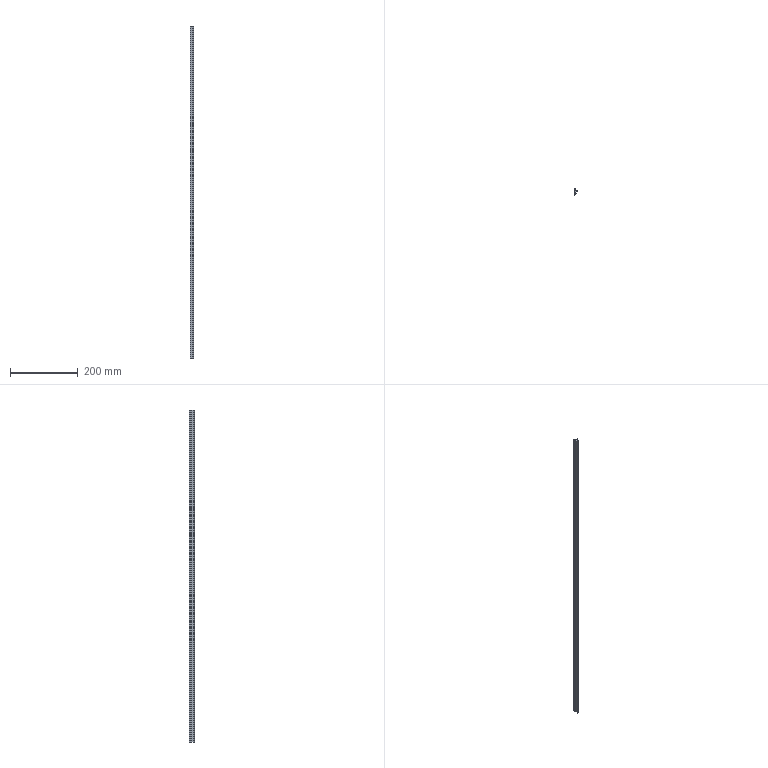Part | SolidWorks | features BaseBody 1, MoveFace 1 | 1 solid | 20 faces | box 10.8 x 17.5 x 980 mm | volume 77225 mm3 | cylinder 11 | plane 9 | commonest cylinder face diameters 1.6 x2 14 x2 0.4 x1 0.6 x1 0.8 x1 2.6 x1
STEP:
#1=CARTESIAN_POINT('',(-3.236,-11.055,880.));
#2=VERTEX_POINT('',#1);
#3=CARTESIAN_POINT('',(-4.3,-10.3,880.));
#4=VERTEX_POINT('',#3);
#5=CARTESIAN_POINT('',(-3.5,-10.3,880.));
#6=DIRECTION('',(0.,0.,-1.));
#7=DIRECTION('',(1.,0.,0.));
#8=AXIS2_PLACEMENT_3D('',#5,#6,#7);
#9=CIRCLE('',#8,0.8);
#10=EDGE_CURVE('',#2,#4,#9,.T.);
#11=ORIENTED_EDGE('',*,*,#10,.T.);
#12=CARTESIAN_POINT('',(-4.3,-10.3,-100.));
#13=VERTEX_POINT('',#12);
#14=CARTESIAN_POINT('',(-4.3,-10.3,-100.));
#15=DIRECTION('',(0.,0.,-1.));
#16=VECTOR('',#15,1000.);
#17=LINE('',#14,#16);
#18=EDGE_CURVE('',#4,#13,#17,.T.);
#19=ORIENTED_EDGE('',*,*,#18,.T.);
#20=CARTESIAN_POINT('',(-3.236,-11.055,-100.));
#21=VERTEX_POINT('',#20);
#22=CARTESIAN_POINT('',(-3.5,-10.3,-100.));
#23=DIRECTION('',(0.,0.,1.));
#24=DIRECTION('',(-1.,0.,0.));
#25=AXIS2_PLACEMENT_3D('',#22,#23,#24);
#26=CIRCLE('',#25,0.8);
#27=EDGE_CURVE('',#13,#21,#26,.T.);
#28=ORIENTED_EDGE('',*,*,#27,.T.);
#29=CARTESIAN_POINT('',(-3.236,-11.055,-100.));
#30=DIRECTION('',(0.,0.,-1.));
#31=VECTOR('',#30,1000.);
#32=LINE('',#29,#31);
#33=EDGE_CURVE('',#2,#21,#32,.T.);
#34=ORIENTED_EDGE('',*,*,#33,.F.);
#35=EDGE_LOOP('',(#11,#19,#28,#34));
#36=FACE_OUTER_BOUND('',#35,.T.);
#37=CARTESIAN_POINT('',(-3.5,-10.3,-100.));
#38=DIRECTION('',(0.,0.,-1.));
#39=DIRECTION('',(-1.,0.,0.));
#40=AXIS2_PLACEMENT_3D('',#37,#38,#39);
#41=CYLINDRICAL_SURFACE('',#40,0.8);
#42=ADVANCED_FACE('',(#36),#41,.T.);
#43=CARTESIAN_POINT('',(1.184,-6.397,-100.));
#44=VERTEX_POINT('',#43);
#45=CARTESIAN_POINT('',(-5.702,-4.29,-100.));
#46=DIRECTION('',(0.,0.,1.));
#47=DIRECTION('',(-1.,0.,0.));
#48=AXIS2_PLACEMENT_3D('',#45,#46,#47);
#49=CIRCLE('',#48,7.201);
#50=EDGE_CURVE('',#21,#44,#49,.T.);
#51=ORIENTED_EDGE('',*,*,#50,.T.);
#52=CARTESIAN_POINT('',(1.184,-6.397,880.));
#53=VERTEX_POINT('',#52);
#54=CARTESIAN_POINT('',(1.184,-6.397,-100.));
#55=DIRECTION('',(0.,0.,1.));
#56=VECTOR('',#55,1000.);
#57=LINE('',#54,#56);
#58=EDGE_CURVE('',#44,#53,#57,.T.);
#59=ORIENTED_EDGE('',*,*,#58,.T.);
#60=CARTESIAN_POINT('',(-5.702,-4.29,880.));
#61=DIRECTION('',(0.,0.,-1.));
#62=DIRECTION('',(1.,0.,0.));
#63=AXIS2_PLACEMENT_3D('',#60,#61,#62);
#64=CIRCLE('',#63,7.201);
#65=EDGE_CURVE('',#53,#2,#64,.T.);
#66=ORIENTED_EDGE('',*,*,#65,.T.);
#67=ORIENTED_EDGE('',*,*,#33,.T.);
#68=EDGE_LOOP('',(#51,#59,#66,#67));
#69=FACE_OUTER_BOUND('',#68,.T.);
#70=CARTESIAN_POINT('',(-5.702,-4.29,-100.));
#71=DIRECTION('',(0.,0.,-1.));
#72=DIRECTION('',(-1.,0.,0.));
#73=AXIS2_PLACEMENT_3D('',#70,#71,#72);
#74=CYLINDRICAL_SURFACE('',#73,7.201);
#75=ADVANCED_FACE('',(#69),#74,.T.);
#76=CARTESIAN_POINT('',(0.9,-6.,-100.));
#77=VERTEX_POINT('',#76);
#78=CARTESIAN_POINT('',(0.9,-6.3,-100.));
#79=DIRECTION('',(0.,0.,1.));
#80=DIRECTION('',(-1.,0.,0.));
#81=AXIS2_PLACEMENT_3D('',#78,#79,#80);
#82=CIRCLE('',#81,0.3);
#83=EDGE_CURVE('',#44,#77,#82,.T.);
#84=ORIENTED_EDGE('',*,*,#83,.T.);
#85=CARTESIAN_POINT('',(0.9,-6.,880.));
#86=VERTEX_POINT('',#85);
#87=CARTESIAN_POINT('',(0.9,-6.,-100.));
#88=DIRECTION('',(0.,0.,1.));
#89=VECTOR('',#88,1000.);
#90=LINE('',#87,#89);
#91=EDGE_CURVE('',#77,#86,#90,.T.);
#92=ORIENTED_EDGE('',*,*,#91,.T.);
#93=CARTESIAN_POINT('',(0.9,-6.3,880.));
#94=DIRECTION('',(0.,0.,-1.));
#95=DIRECTION('',(1.,0.,0.));
#96=AXIS2_PLACEMENT_3D('',#93,#94,#95);
#97=CIRCLE('',#96,0.3);
#98=EDGE_CURVE('',#86,#53,#97,.T.);
#99=ORIENTED_EDGE('',*,*,#98,.T.);
#100=ORIENTED_EDGE('',*,*,#58,.F.);
#101=EDGE_LOOP('',(#84,#92,#99,#100));
#102=FACE_OUTER_BOUND('',#101,.T.);
#103=CARTESIAN_POINT('',(0.9,-6.3,-100.));
#104=DIRECTION('',(0.,0.,-1.));
#105=DIRECTION('',(-1.,0.,0.));
#106=AXIS2_PLACEMENT_3D('',#103,#104,#105);
#107=CYLINDRICAL_SURFACE('',#106,0.3);
#108=ADVANCED_FACE('',(#102),#107,.T.);
#109=CARTESIAN_POINT('',(-2.5,-0.5,-100.));
#110=VERTEX_POINT('',#109);
#111=CARTESIAN_POINT('',(-2.5,-6.153,-100.));
#112=VERTEX_POINT('',#111);
#113=CARTESIAN_POINT('',(-2.5,-6.397,-100.));
#114=DIRECTION('',(0.,-1.,0.));
#115=VECTOR('',#114,1000.);
#116=LINE('',#113,#115);
#117=EDGE_CURVE('',#110,#112,#116,.T.);
#118=ORIENTED_EDGE('',*,*,#117,.F.);
#119=CARTESIAN_POINT('',(-4.2,1.695,-100.));
#120=VERTEX_POINT('',#119);
#121=CARTESIAN_POINT('',(-1.701,1.875,-100.));
#122=DIRECTION('',(0.,0.,1.));
#123=DIRECTION('',(-1.,0.,0.));
#124=AXIS2_PLACEMENT_3D('',#121,#122,#123);
#125=CIRCLE('',#124,2.506);
#126=EDGE_CURVE('',#120,#110,#125,.T.);
#127=ORIENTED_EDGE('',*,*,#126,.F.);
#128=CARTESIAN_POINT('',(-4.2,5.1,-100.));
#129=VERTEX_POINT('',#128);
#130=CARTESIAN_POINT('',(-4.2,-6.397,-100.));
#131=DIRECTION('',(0.,-1.,0.));
#132=VECTOR('',#131,1000.);
#133=LINE('',#130,#132);
#134=EDGE_CURVE('',#129,#120,#133,.T.);
#135=ORIENTED_EDGE('',*,*,#134,.F.);
#136=CARTESIAN_POINT('',(-2.892,6.4,-100.));
#137=VERTEX_POINT('',#136);
#138=CARTESIAN_POINT('',(-2.9,5.1,-100.));
#139=DIRECTION('',(0.,0.,1.));
#140=DIRECTION('',(-1.,0.,0.));
#141=AXIS2_PLACEMENT_3D('',#138,#139,#140);
#142=CIRCLE('',#141,1.3);
#143=EDGE_CURVE('',#137,#129,#142,.T.);
#144=ORIENTED_EDGE('',*,*,#143,.F.);
#145=CARTESIAN_POINT('',(0.5,5.5,-100.));
#146=VERTEX_POINT('',#145);
#147=CARTESIAN_POINT('',(-2.934,-0.5999,-100.));
#148=DIRECTION('',(0.,0.,1.));
#149=DIRECTION('',(-1.,0.,0.));
#150=AXIS2_PLACEMENT_3D('',#147,#148,#149);
#151=CIRCLE('',#150,7.);
#152=EDGE_CURVE('',#146,#137,#151,.T.);
#153=ORIENTED_EDGE('',*,*,#152,.F.);
#154=CARTESIAN_POINT('',(5.5,1.7,-100.));
#155=VERTEX_POINT('',#154);
#156=CARTESIAN_POINT('',(5.5,1.7,-100.));
#157=DIRECTION('',(-0.7962,0.6051,0.));
#158=VECTOR('',#157,1000.);
#159=LINE('',#156,#158);
#160=EDGE_CURVE('',#155,#146,#159,.T.);
#161=ORIENTED_EDGE('',*,*,#160,.F.);
#162=CARTESIAN_POINT('',(6.458,-0.2215,-100.));
#163=VERTEX_POINT('',#162);
#164=CARTESIAN_POINT('',(6.458,-0.2215,-100.));
#165=DIRECTION('',(-0.4462,0.8949,0.));
#166=VECTOR('',#165,1000.);
#167=LINE('',#164,#166);
#168=EDGE_CURVE('',#163,#155,#167,.T.);
#169=ORIENTED_EDGE('',*,*,#168,.F.);
#170=CARTESIAN_POINT('',(5.895,-0.7433,-100.));
#171=VERTEX_POINT('',#170);
#172=CARTESIAN_POINT('',(6.1,-0.4,-100.));
#173=DIRECTION('',(0.,0.,1.));
#174=DIRECTION('',(-1.,0.,0.));
#175=AXIS2_PLACEMENT_3D('',#172,#173,#174);
#176=CIRCLE('',#175,0.4);
#177=EDGE_CURVE('',#171,#163,#176,.T.);
#178=ORIENTED_EDGE('',*,*,#177,.F.);
#179=CARTESIAN_POINT('',(3.,0.,-100.));
#180=VERTEX_POINT('',#179);
#181=CARTESIAN_POINT('',(2.746,-6.995,-100.));
#182=DIRECTION('',(0.,0.,-1.));
#183=DIRECTION('',(-1.,0.,0.));
#184=AXIS2_PLACEMENT_3D('',#181,#182,#183);
#185=CIRCLE('',#184,7.);
#186=EDGE_CURVE('',#180,#171,#185,.T.);
#187=ORIENTED_EDGE('',*,*,#186,.F.);
#188=CARTESIAN_POINT('',(0.,0.,-100.));
#189=VERTEX_POINT('',#188);
#190=CARTESIAN_POINT('',(-6.814,0.,-100.));
#191=DIRECTION('',(1.,0.,0.));
#192=VECTOR('',#191,1000.);
#193=LINE('',#190,#192);
#194=EDGE_CURVE('',#189,#180,#193,.T.);
#195=ORIENTED_EDGE('',*,*,#194,.F.);
#196=CARTESIAN_POINT('',(0.,-5.8,-100.));
#197=VERTEX_POINT('',#196);
#198=CARTESIAN_POINT('',(0.,-6.397,-100.));
#199=DIRECTION('',(0.,1.,0.));
#200=VECTOR('',#199,1000.);
#201=LINE('',#198,#200);
#202=EDGE_CURVE('',#197,#189,#201,.T.);
#203=ORIENTED_EDGE('',*,*,#202,.F.);
#204=CARTESIAN_POINT('',(0.2,-6.,-100.));
#205=VERTEX_POINT('',#204);
#206=CARTESIAN_POINT('',(0.2,-5.8,-100.));
#207=DIRECTION('',(0.,0.,1.));
#208=DIRECTION('',(-1.,0.,0.));
#209=AXIS2_PLACEMENT_3D('',#206,#207,#208);
#210=CIRCLE('',#209,0.2);
#211=EDGE_CURVE('',#197,#205,#210,.T.);
#212=ORIENTED_EDGE('',*,*,#211,.T.);
#213=CARTESIAN_POINT('',(-6.814,-6.,-100.));
#214=DIRECTION('',(-1.,0.,0.));
#215=VECTOR('',#214,1000.);
#216=LINE('',#213,#215);
#217=EDGE_CURVE('',#77,#205,#216,.T.);
#218=ORIENTED_EDGE('',*,*,#217,.F.);
#219=ORIENTED_EDGE('',*,*,#83,.F.);
#220=ORIENTED_EDGE('',*,*,#50,.F.);
#221=ORIENTED_EDGE('',*,*,#27,.F.);
#222=CARTESIAN_POINT('',(-3.998,-9.674,-100.));
#223=VERTEX_POINT('',#222);
#224=CARTESIAN_POINT('',(-3.5,-10.3,-100.));
#225=DIRECTION('',(0.,0.,1.));
#226=DIRECTION('',(-1.,0.,0.));
#227=AXIS2_PLACEMENT_3D('',#224,#225,#226);
#228=CIRCLE('',#227,0.8);
#229=EDGE_CURVE('',#223,#13,#228,.T.);
#230=ORIENTED_EDGE('',*,*,#229,.F.);
#231=CARTESIAN_POINT('',(-6.814,-6.397,-100.));
#232=DIRECTION('',(0.,0.,-1.));
#233=DIRECTION('',(-1.,0.,0.));
#234=AXIS2_PLACEMENT_3D('',#231,#232,#233);
#235=CIRCLE('',#234,4.321);
#236=EDGE_CURVE('',#112,#223,#235,.T.);
#237=ORIENTED_EDGE('',*,*,#236,.F.);
#238=EDGE_LOOP('',(#118,#127,#135,#144,#153,#161,#169,#178,#187,#195,#203,#212,#218,#219,#220,#221,#230,#237));
#239=FACE_OUTER_BOUND('',#238,.T.);
#240=CARTESIAN_POINT('',(-6.814,-6.397,-100.));
#241=DIRECTION('',(0.,0.,1.));
#242=DIRECTION('',(1.,0.,0.));
#243=AXIS2_PLACEMENT_3D('',#240,#241,#242);
#244=PLANE('',#243);
#245=ADVANCED_FACE('',(#239),#244,.F.);
#246=ORIENTED_EDGE('',*,*,#18,.F.);
#247=CARTESIAN_POINT('',(-3.998,-9.674,880.));
#248=VERTEX_POINT('',#247);
#249=CARTESIAN_POINT('',(-3.5,-10.3,880.));
#250=DIRECTION('',(0.,0.,-1.));
#251=DIRECTION('',(1.,0.,0.));
#252=AXIS2_PLACEMENT_3D('',#249,#250,#251);
#253=CIRCLE('',#252,0.8);
#254=EDGE_CURVE('',#4,#248,#253,.T.);
#255=ORIENTED_EDGE('',*,*,#254,.T.);
#256=CARTESIAN_POINT('',(-3.998,-9.674,-100.));
#257=DIRECTION('',(0.,0.,-1.));
#258=VECTOR('',#257,1000.);
#259=LINE('',#256,#258);
#260=EDGE_CURVE('',#248,#223,#259,.T.);
#261=ORIENTED_EDGE('',*,*,#260,.T.);
#262=ORIENTED_EDGE('',*,*,#229,.T.);
#263=EDGE_LOOP('',(#246,#255,#261,#262));
#264=FACE_OUTER_BOUND('',#263,.T.);
#265=CARTESIAN_POINT('',(-3.5,-10.3,-100.));
#266=DIRECTION('',(0.,0.,-1.));
#267=DIRECTION('',(-1.,0.,0.));
#268=AXIS2_PLACEMENT_3D('',#265,#266,#267);
#269=CYLINDRICAL_SURFACE('',#268,0.8);
#270=ADVANCED_FACE('',(#264),#269,.T.);
#271=CARTESIAN_POINT('',(-4.2,1.695,880.));
#272=VERTEX_POINT('',#271);
#273=CARTESIAN_POINT('',(-2.5,-0.5,880.));
#274=VERTEX_POINT('',#273);
#275=CARTESIAN_POINT('',(-1.701,1.875,880.));
#276=DIRECTION('',(0.,0.,1.));
#277=DIRECTION('',(1.,0.,0.));
#278=AXIS2_PLACEMENT_3D('',#275,#276,#277);
#279=CIRCLE('',#278,2.506);
#280=EDGE_CURVE('',#272,#274,#279,.T.);
#281=ORIENTED_EDGE('',*,*,#280,.T.);
#282=CARTESIAN_POINT('',(-2.5,-6.153,880.));
#283=VERTEX_POINT('',#282);
#284=CARTESIAN_POINT('',(-2.5,-6.397,880.));
#285=DIRECTION('',(0.,-1.,0.));
#286=VECTOR('',#285,1000.);
#287=LINE('',#284,#286);
#288=EDGE_CURVE('',#274,#283,#287,.T.);
#289=ORIENTED_EDGE('',*,*,#288,.T.);
#290=CARTESIAN_POINT('',(-6.814,-6.397,880.));
#291=DIRECTION('',(0.,0.,-1.));
#292=DIRECTION('',(1.,0.,0.));
#293=AXIS2_PLACEMENT_3D('',#290,#291,#292);
#294=CIRCLE('',#293,4.321);
#295=EDGE_CURVE('',#283,#248,#294,.T.);
#296=ORIENTED_EDGE('',*,*,#295,.T.);
#297=ORIENTED_EDGE('',*,*,#254,.F.);
#298=ORIENTED_EDGE('',*,*,#10,.F.);
#299=ORIENTED_EDGE('',*,*,#65,.F.);
#300=ORIENTED_EDGE('',*,*,#98,.F.);
#301=CARTESIAN_POINT('',(0.2,-6.,880.));
#302=VERTEX_POINT('',#301);
#303=CARTESIAN_POINT('',(-6.814,-6.,880.));
#304=DIRECTION('',(-1.,0.,0.));
#305=VECTOR('',#304,1000.);
#306=LINE('',#303,#305);
#307=EDGE_CURVE('',#86,#302,#306,.T.);
#308=ORIENTED_EDGE('',*,*,#307,.T.);
#309=CARTESIAN_POINT('',(0.,-5.8,880.));
#310=VERTEX_POINT('',#309);
#311=CARTESIAN_POINT('',(0.2,-5.8,880.));
#312=DIRECTION('',(0.,0.,-1.));
#313=DIRECTION('',(1.,0.,0.));
#314=AXIS2_PLACEMENT_3D('',#311,#312,#313);
#315=CIRCLE('',#314,0.2);
#316=EDGE_CURVE('',#302,#310,#315,.T.);
#317=ORIENTED_EDGE('',*,*,#316,.T.);
#318=CARTESIAN_POINT('',(0.,0.,880.));
#319=VERTEX_POINT('',#318);
#320=CARTESIAN_POINT('',(0.,-6.397,880.));
#321=DIRECTION('',(0.,1.,0.));
#322=VECTOR('',#321,1000.);
#323=LINE('',#320,#322);
#324=EDGE_CURVE('',#310,#319,#323,.T.);
#325=ORIENTED_EDGE('',*,*,#324,.T.);
#326=CARTESIAN_POINT('',(3.,0.,880.));
#327=VERTEX_POINT('',#326);
#328=CARTESIAN_POINT('',(-6.814,0.,880.));
#329=DIRECTION('',(1.,0.,0.));
#330=VECTOR('',#329,1000.);
#331=LINE('',#328,#330);
#332=EDGE_CURVE('',#319,#327,#331,.T.);
#333=ORIENTED_EDGE('',*,*,#332,.T.);
#334=CARTESIAN_POINT('',(5.895,-0.7433,880.));
#335=VERTEX_POINT('',#334);
#336=CARTESIAN_POINT('',(2.746,-6.995,880.));
#337=DIRECTION('',(0.,0.,-1.));
#338=DIRECTION('',(1.,0.,0.));
#339=AXIS2_PLACEMENT_3D('',#336,#337,#338);
#340=CIRCLE('',#339,7.);
#341=EDGE_CURVE('',#327,#335,#340,.T.);
#342=ORIENTED_EDGE('',*,*,#341,.T.);
#343=CARTESIAN_POINT('',(6.458,-0.2215,880.));
#344=VERTEX_POINT('',#343);
#345=CARTESIAN_POINT('',(6.1,-0.4,880.));
#346=DIRECTION('',(0.,0.,-1.));
#347=DIRECTION('',(1.,0.,0.));
#348=AXIS2_PLACEMENT_3D('',#345,#346,#347);
#349=CIRCLE('',#348,0.4);
#350=EDGE_CURVE('',#344,#335,#349,.T.);
#351=ORIENTED_EDGE('',*,*,#350,.F.);
#352=CARTESIAN_POINT('',(5.5,1.7,880.));
#353=VERTEX_POINT('',#352);
#354=CARTESIAN_POINT('',(6.282,0.1323,880.));
#355=DIRECTION('',(-0.4462,0.8949,0.));
#356=VECTOR('',#355,1000.);
#357=LINE('',#354,#356);
#358=EDGE_CURVE('',#344,#353,#357,.T.);
#359=ORIENTED_EDGE('',*,*,#358,.T.);
#360=CARTESIAN_POINT('',(0.5,5.5,880.));
#361=VERTEX_POINT('',#360);
#362=CARTESIAN_POINT('',(1.595,4.668,880.));
#363=DIRECTION('',(-0.7962,0.6051,0.));
#364=VECTOR('',#363,1000.);
#365=LINE('',#362,#364);
#366=EDGE_CURVE('',#353,#361,#365,.T.);
#367=ORIENTED_EDGE('',*,*,#366,.T.);
#368=CARTESIAN_POINT('',(-2.892,6.4,880.));
#369=VERTEX_POINT('',#368);
#370=CARTESIAN_POINT('',(-2.934,-0.5999,880.));
#371=DIRECTION('',(0.,0.,1.));
#372=DIRECTION('',(1.,0.,0.));
#373=AXIS2_PLACEMENT_3D('',#370,#371,#372);
#374=CIRCLE('',#373,7.);
#375=EDGE_CURVE('',#361,#369,#374,.T.);
#376=ORIENTED_EDGE('',*,*,#375,.T.);
#377=CARTESIAN_POINT('',(-4.2,5.1,880.));
#378=VERTEX_POINT('',#377);
#379=CARTESIAN_POINT('',(-2.9,5.1,880.));
#380=DIRECTION('',(0.,0.,1.));
#381=DIRECTION('',(1.,0.,0.));
#382=AXIS2_PLACEMENT_3D('',#379,#380,#381);
#383=CIRCLE('',#382,1.3);
#384=EDGE_CURVE('',#369,#378,#383,.T.);
#385=ORIENTED_EDGE('',*,*,#384,.T.);
#386=CARTESIAN_POINT('',(-4.2,-6.397,880.));
#387=DIRECTION('',(0.,-1.,0.));
#388=VECTOR('',#387,1000.);
#389=LINE('',#386,#388);
#390=EDGE_CURVE('',#378,#272,#389,.T.);
#391=ORIENTED_EDGE('',*,*,#390,.T.);
#392=EDGE_LOOP('',(#281,#289,#296,#297,#298,#299,#300,#308,#317,#325,#333,#342,#351,#359,#367,#376,#385,#391));
#393=FACE_OUTER_BOUND('',#392,.T.);
#394=CARTESIAN_POINT('',(-6.814,-6.397,880.));
#395=DIRECTION('',(0.,0.,1.));
#396=DIRECTION('',(1.,0.,0.));
#397=AXIS2_PLACEMENT_3D('',#394,#395,#396);
#398=PLANE('',#397);
#399=ADVANCED_FACE('',(#393),#398,.T.);
#400=ORIENTED_EDGE('',*,*,#217,.T.);
#401=CARTESIAN_POINT('',(0.2,-6.,-100.));
#402=DIRECTION('',(0.,0.,1.));
#403=VECTOR('',#402,1000.);
#404=LINE('',#401,#403);
#405=EDGE_CURVE('',#205,#302,#404,.T.);
#406=ORIENTED_EDGE('',*,*,#405,.T.);
#407=ORIENTED_EDGE('',*,*,#307,.F.);
#408=ORIENTED_EDGE('',*,*,#91,.F.);
#409=EDGE_LOOP('',(#400,#406,#407,#408));
#410=FACE_OUTER_BOUND('',#409,.T.);
#411=CARTESIAN_POINT('',(0.9,-6.,-100.));
#412=DIRECTION('',(0.,1.,0.));
#413=DIRECTION('',(0.,0.,1.));
#414=AXIS2_PLACEMENT_3D('',#411,#412,#413);
#415=PLANE('',#414);
#416=ADVANCED_FACE('',(#410),#415,.T.);
#417=CARTESIAN_POINT('',(-2.5,-6.153,-100.));
#418=DIRECTION('',(0.,0.,1.));
#419=VECTOR('',#418,1000.);
#420=LINE('',#417,#419);
#421=EDGE_CURVE('',#112,#283,#420,.T.);
#422=ORIENTED_EDGE('',*,*,#421,.F.);
#423=ORIENTED_EDGE('',*,*,#236,.T.);
#424=ORIENTED_EDGE('',*,*,#260,.F.);
#425=ORIENTED_EDGE('',*,*,#295,.F.);
#426=EDGE_LOOP('',(#422,#423,#424,#425));
#427=FACE_OUTER_BOUND('',#426,.T.);
#428=CARTESIAN_POINT('',(-6.814,-6.397,-100.));
#429=DIRECTION('',(0.,0.,-1.));
#430=DIRECTION('',(-1.,0.,0.));
#431=AXIS2_PLACEMENT_3D('',#428,#429,#430);
#432=CYLINDRICAL_SURFACE('',#431,4.321);
#433=ADVANCED_FACE('',(#427),#432,.F.);
#434=ORIENTED_EDGE('',*,*,#117,.T.);
#435=ORIENTED_EDGE('',*,*,#421,.T.);
#436=ORIENTED_EDGE('',*,*,#288,.F.);
#437=CARTESIAN_POINT('',(-2.5,-0.5,-100.));
#438=DIRECTION('',(0.,0.,-1.));
#439=VECTOR('',#438,1000.);
#440=LINE('',#437,#439);
#441=EDGE_CURVE('',#274,#110,#440,.T.);
#442=ORIENTED_EDGE('',*,*,#441,.T.);
#443=EDGE_LOOP('',(#434,#435,#436,#442));
#444=FACE_OUTER_BOUND('',#443,.T.);
#445=CARTESIAN_POINT('',(-2.5,-0.5,-100.));
#446=DIRECTION('',(-1.,0.,0.));
#447=DIRECTION('',(0.,0.,1.));
#448=AXIS2_PLACEMENT_3D('',#445,#446,#447);
#449=PLANE('',#448);
#450=ADVANCED_FACE('',(#444),#449,.T.);
#451=ORIENTED_EDGE('',*,*,#126,.T.);
#452=ORIENTED_EDGE('',*,*,#441,.F.);
#453=ORIENTED_EDGE('',*,*,#280,.F.);
#454=CARTESIAN_POINT('',(-4.2,1.695,-100.));
#455=DIRECTION('',(0.,0.,-1.));
#456=VECTOR('',#455,1000.);
#457=LINE('',#454,#456);
#458=EDGE_CURVE('',#272,#120,#457,.T.);
#459=ORIENTED_EDGE('',*,*,#458,.T.);
#460=EDGE_LOOP('',(#451,#452,#453,#459));
#461=FACE_OUTER_BOUND('',#460,.T.);
#462=CARTESIAN_POINT('',(-1.701,1.875,-100.));
#463=DIRECTION('',(0.,0.,-1.));
#464=DIRECTION('',(-1.,0.,0.));
#465=AXIS2_PLACEMENT_3D('',#462,#463,#464);
#466=CYLINDRICAL_SURFACE('',#465,2.506);
#467=ADVANCED_FACE('',(#461),#466,.T.);
#468=ORIENTED_EDGE('',*,*,#134,.T.);
#469=ORIENTED_EDGE('',*,*,#458,.F.);
#470=ORIENTED_EDGE('',*,*,#390,.F.);
#471=CARTESIAN_POINT('',(-4.2,5.1,-100.));
#472=DIRECTION('',(0.,0.,-1.));
#473=VECTOR('',#472,1000.);
#474=LINE('',#471,#473);
#475=EDGE_CURVE('',#378,#129,#474,.T.);
#476=ORIENTED_EDGE('',*,*,#475,.T.);
#477=EDGE_LOOP('',(#468,#469,#470,#476));
#478=FACE_OUTER_BOUND('',#477,.T.);
#479=CARTESIAN_POINT('',(-4.2,5.1,-100.));
#480=DIRECTION('',(-1.,0.,0.));
#481=DIRECTION('',(0.,0.,1.));
#482=AXIS2_PLACEMENT_3D('',#479,#480,#481);
#483=PLANE('',#482);
#484=ADVANCED_FACE('',(#478),#483,.T.);
#485=ORIENTED_EDGE('',*,*,#143,.T.);
#486=ORIENTED_EDGE('',*,*,#475,.F.);
#487=ORIENTED_EDGE('',*,*,#384,.F.);
#488=CARTESIAN_POINT('',(-2.892,6.4,-100.));
#489=DIRECTION('',(0.,0.,-1.));
#490=VECTOR('',#489,1000.);
#491=LINE('',#488,#490);
#492=EDGE_CURVE('',#369,#137,#491,.T.);
#493=ORIENTED_EDGE('',*,*,#492,.T.);
#494=EDGE_LOOP('',(#485,#486,#487,#493));
#495=FACE_OUTER_BOUND('',#494,.T.);
#496=CARTESIAN_POINT('',(-2.9,5.1,-100.));
#497=DIRECTION('',(0.,0.,-1.));
#498=DIRECTION('',(-1.,0.,0.));
#499=AXIS2_PLACEMENT_3D('',#496,#497,#498);
#500=CYLINDRICAL_SURFACE('',#499,1.3);
#501=ADVANCED_FACE('',(#495),#500,.T.);
#502=ORIENTED_EDGE('',*,*,#152,.T.);
#503=ORIENTED_EDGE('',*,*,#492,.F.);
#504=ORIENTED_EDGE('',*,*,#375,.F.);
#505=CARTESIAN_POINT('',(0.5,5.5,-100.));
#506=DIRECTION('',(0.,0.,-1.));
#507=VECTOR('',#506,1000.);
#508=LINE('',#505,#507);
#509=EDGE_CURVE('',#361,#146,#508,.T.);
#510=ORIENTED_EDGE('',*,*,#509,.T.);
#511=EDGE_LOOP('',(#502,#503,#504,#510));
#512=FACE_OUTER_BOUND('',#511,.T.);
#513=CARTESIAN_POINT('',(-2.934,-0.5999,-100.));
#514=DIRECTION('',(0.,0.,-1.));
#515=DIRECTION('',(-1.,0.,0.));
#516=AXIS2_PLACEMENT_3D('',#513,#514,#515);
#517=CYLINDRICAL_SURFACE('',#516,7.);
#518=ADVANCED_FACE('',(#512),#517,.T.);
#519=ORIENTED_EDGE('',*,*,#160,.T.);
#520=ORIENTED_EDGE('',*,*,#509,.F.);
#521=ORIENTED_EDGE('',*,*,#366,.F.);
#522=CARTESIAN_POINT('',(5.5,1.7,-100.));
#523=DIRECTION('',(0.,0.,-1.));
#524=VECTOR('',#523,1000.);
#525=LINE('',#522,#524);
#526=EDGE_CURVE('',#353,#155,#525,.T.);
#527=ORIENTED_EDGE('',*,*,#526,.T.);
#528=EDGE_LOOP('',(#519,#520,#521,#527));
#529=FACE_OUTER_BOUND('',#528,.T.);
#530=CARTESIAN_POINT('',(5.5,1.7,-100.));
#531=DIRECTION('',(0.6051,0.7962,0.));
#532=DIRECTION('',(-0.7962,0.6051,0.));
#533=AXIS2_PLACEMENT_3D('',#530,#531,#532);
#534=PLANE('',#533);
#535=ADVANCED_FACE('',(#529),#534,.T.);
#536=ORIENTED_EDGE('',*,*,#168,.T.);
#537=ORIENTED_EDGE('',*,*,#526,.F.);
#538=ORIENTED_EDGE('',*,*,#358,.F.);
#539=CARTESIAN_POINT('',(6.458,-0.2215,-100.));
#540=DIRECTION('',(0.,0.,-1.));
#541=VECTOR('',#540,1000.);
#542=LINE('',#539,#541);
#543=EDGE_CURVE('',#344,#163,#542,.T.);
#544=ORIENTED_EDGE('',*,*,#543,.T.);
#545=EDGE_LOOP('',(#536,#537,#538,#544));
#546=FACE_OUTER_BOUND('',#545,.T.);
#547=CARTESIAN_POINT('',(6.458,-0.2215,-100.));
#548=DIRECTION('',(0.8949,0.4462,0.));
#549=DIRECTION('',(-0.4462,0.8949,0.));
#550=AXIS2_PLACEMENT_3D('',#547,#548,#549);
#551=PLANE('',#550);
#552=ADVANCED_FACE('',(#546),#551,.T.);
#553=CARTESIAN_POINT('',(3.,0.,-100.));
#554=DIRECTION('',(0.,0.,1.));
#555=VECTOR('',#554,1000.);
#556=LINE('',#553,#555);
#557=EDGE_CURVE('',#180,#327,#556,.T.);
#558=ORIENTED_EDGE('',*,*,#557,.F.);
#559=ORIENTED_EDGE('',*,*,#186,.T.);
#560=CARTESIAN_POINT('',(5.895,-0.7433,-100.));
#561=DIRECTION('',(0.,0.,-1.));
#562=VECTOR('',#561,1000.);
#563=LINE('',#560,#562);
#564=EDGE_CURVE('',#335,#171,#563,.T.);
#565=ORIENTED_EDGE('',*,*,#564,.F.);
#566=ORIENTED_EDGE('',*,*,#341,.F.);
#567=EDGE_LOOP('',(#558,#559,#565,#566));
#568=FACE_OUTER_BOUND('',#567,.T.);
#569=CARTESIAN_POINT('',(2.746,-6.995,-100.));
#570=DIRECTION('',(0.,0.,-1.));
#571=DIRECTION('',(-1.,0.,0.));
#572=AXIS2_PLACEMENT_3D('',#569,#570,#571);
#573=CYLINDRICAL_SURFACE('',#572,7.);
#574=ADVANCED_FACE('',(#568),#573,.F.);
#575=ORIENTED_EDGE('',*,*,#194,.T.);
#576=ORIENTED_EDGE('',*,*,#557,.T.);
#577=ORIENTED_EDGE('',*,*,#332,.F.);
#578=CARTESIAN_POINT('',(0.,0.,-100.));
#579=DIRECTION('',(0.,0.,-1.));
#580=VECTOR('',#579,1000.);
#581=LINE('',#578,#580);
#582=EDGE_CURVE('',#319,#189,#581,.T.);
#583=ORIENTED_EDGE('',*,*,#582,.T.);
#584=EDGE_LOOP('',(#575,#576,#577,#583));
#585=FACE_OUTER_BOUND('',#584,.T.);
#586=CARTESIAN_POINT('',(0.,0.,-100.));
#587=DIRECTION('',(0.,-1.,0.));
#588=DIRECTION('',(0.,0.,-1.));
#589=AXIS2_PLACEMENT_3D('',#586,#587,#588);
#590=PLANE('',#589);
#591=ADVANCED_FACE('',(#585),#590,.T.);
#592=ORIENTED_EDGE('',*,*,#202,.T.);
#593=ORIENTED_EDGE('',*,*,#582,.F.);
#594=ORIENTED_EDGE('',*,*,#324,.F.);
#595=CARTESIAN_POINT('',(0.,-5.8,-100.));
#596=DIRECTION('',(0.,0.,-1.));
#597=VECTOR('',#596,1000.);
#598=LINE('',#595,#597);
#599=EDGE_CURVE('',#310,#197,#598,.T.);
#600=ORIENTED_EDGE('',*,*,#599,.T.);
#601=EDGE_LOOP('',(#592,#593,#594,#600));
#602=FACE_OUTER_BOUND('',#601,.T.);
#603=CARTESIAN_POINT('',(0.,-5.8,-100.));
#604=DIRECTION('',(1.,0.,0.));
#605=DIRECTION('',(0.,0.,-1.));
#606=AXIS2_PLACEMENT_3D('',#603,#604,#605);
#607=PLANE('',#606);
#608=ADVANCED_FACE('',(#602),#607,.T.);
#609=ORIENTED_EDGE('',*,*,#405,.F.);
#610=ORIENTED_EDGE('',*,*,#211,.F.);
#611=ORIENTED_EDGE('',*,*,#599,.F.);
#612=ORIENTED_EDGE('',*,*,#316,.F.);
#613=EDGE_LOOP('',(#609,#610,#611,#612));
#614=FACE_OUTER_BOUND('',#613,.T.);
#615=CARTESIAN_POINT('',(0.2,-5.8,-100.));
#616=DIRECTION('',(0.,0.,-1.));
#617=DIRECTION('',(-1.,0.,0.));
#618=AXIS2_PLACEMENT_3D('',#615,#616,#617);
#619=CYLINDRICAL_SURFACE('',#618,0.2);
#620=ADVANCED_FACE('',(#614),#619,.F.);
#621=ORIENTED_EDGE('',*,*,#177,.T.);
#622=ORIENTED_EDGE('',*,*,#543,.F.);
#623=ORIENTED_EDGE('',*,*,#350,.T.);
#624=ORIENTED_EDGE('',*,*,#564,.T.);
#625=EDGE_LOOP('',(#621,#622,#623,#624));
#626=FACE_OUTER_BOUND('',#625,.T.);
#627=CARTESIAN_POINT('',(6.1,-0.4,-100.));
#628=DIRECTION('',(0.,0.,-1.));
#629=DIRECTION('',(-1.,0.,0.));
#630=AXIS2_PLACEMENT_3D('',#627,#628,#629);
#631=CYLINDRICAL_SURFACE('',#630,0.4);
#632=ADVANCED_FACE('',(#626),#631,.T.);
#633=CLOSED_SHELL('',(#42,#75,#108,#245,#270,#399,#416,#433,#450,#467,#484,#501,#518,#535,#552,#574,#591,#608,#620,#632));
#634=MANIFOLD_SOLID_BREP('',#633);
#635=CARTESIAN_POINT('',(0.,0.,0.));
#636=DIRECTION('',(0.,0.,1.));
#637=DIRECTION('',(1.,0.,0.));
#638=AXIS2_PLACEMENT_3D('',#635,#636,#637);
#639=(LENGTH_UNIT()NAMED_UNIT(*)SI_UNIT(.MILLI.,.METRE.));
#640=UNCERTAINTY_MEASURE_WITH_UNIT(LENGTH_MEASURE(0.00001),#639,'','');
#641=(NAMED_UNIT(*)PLANE_ANGLE_UNIT()SI_UNIT($,.RADIAN.));
#642=(NAMED_UNIT(*)SI_UNIT($,.STERADIAN.)SOLID_ANGLE_UNIT());
#643=(GEOMETRIC_REPRESENTATION_CONTEXT(3)GLOBAL_UNCERTAINTY_ASSIGNED_CONTEXT((#640))GLOBAL_UNIT_ASSIGNED_CONTEXT((#639,#641,#642))REPRESENTATION_CONTEXT('',''));
#644=ADVANCED_BREP_SHAPE_REPRESENTATION('',(#634,#638),#643);